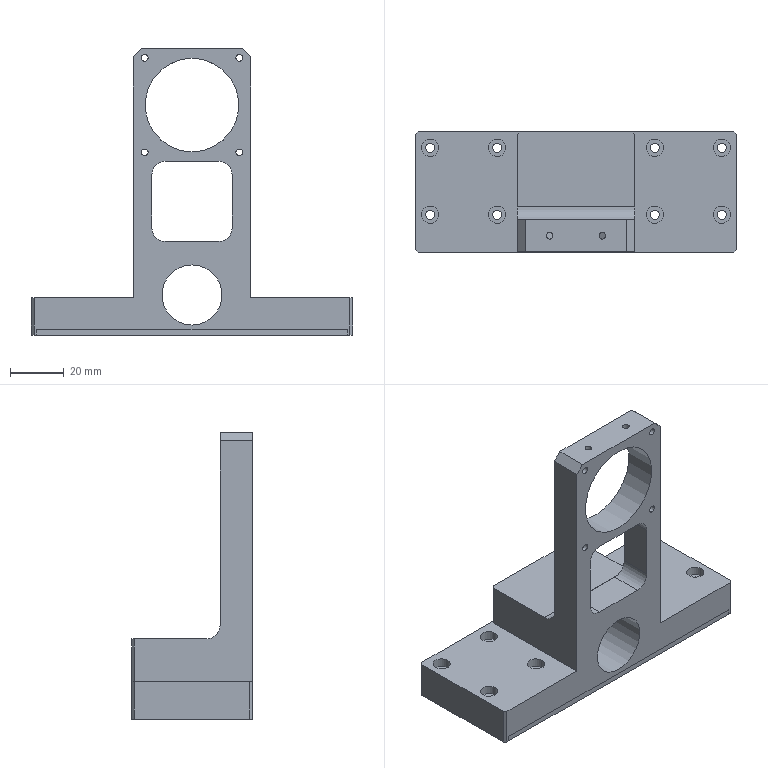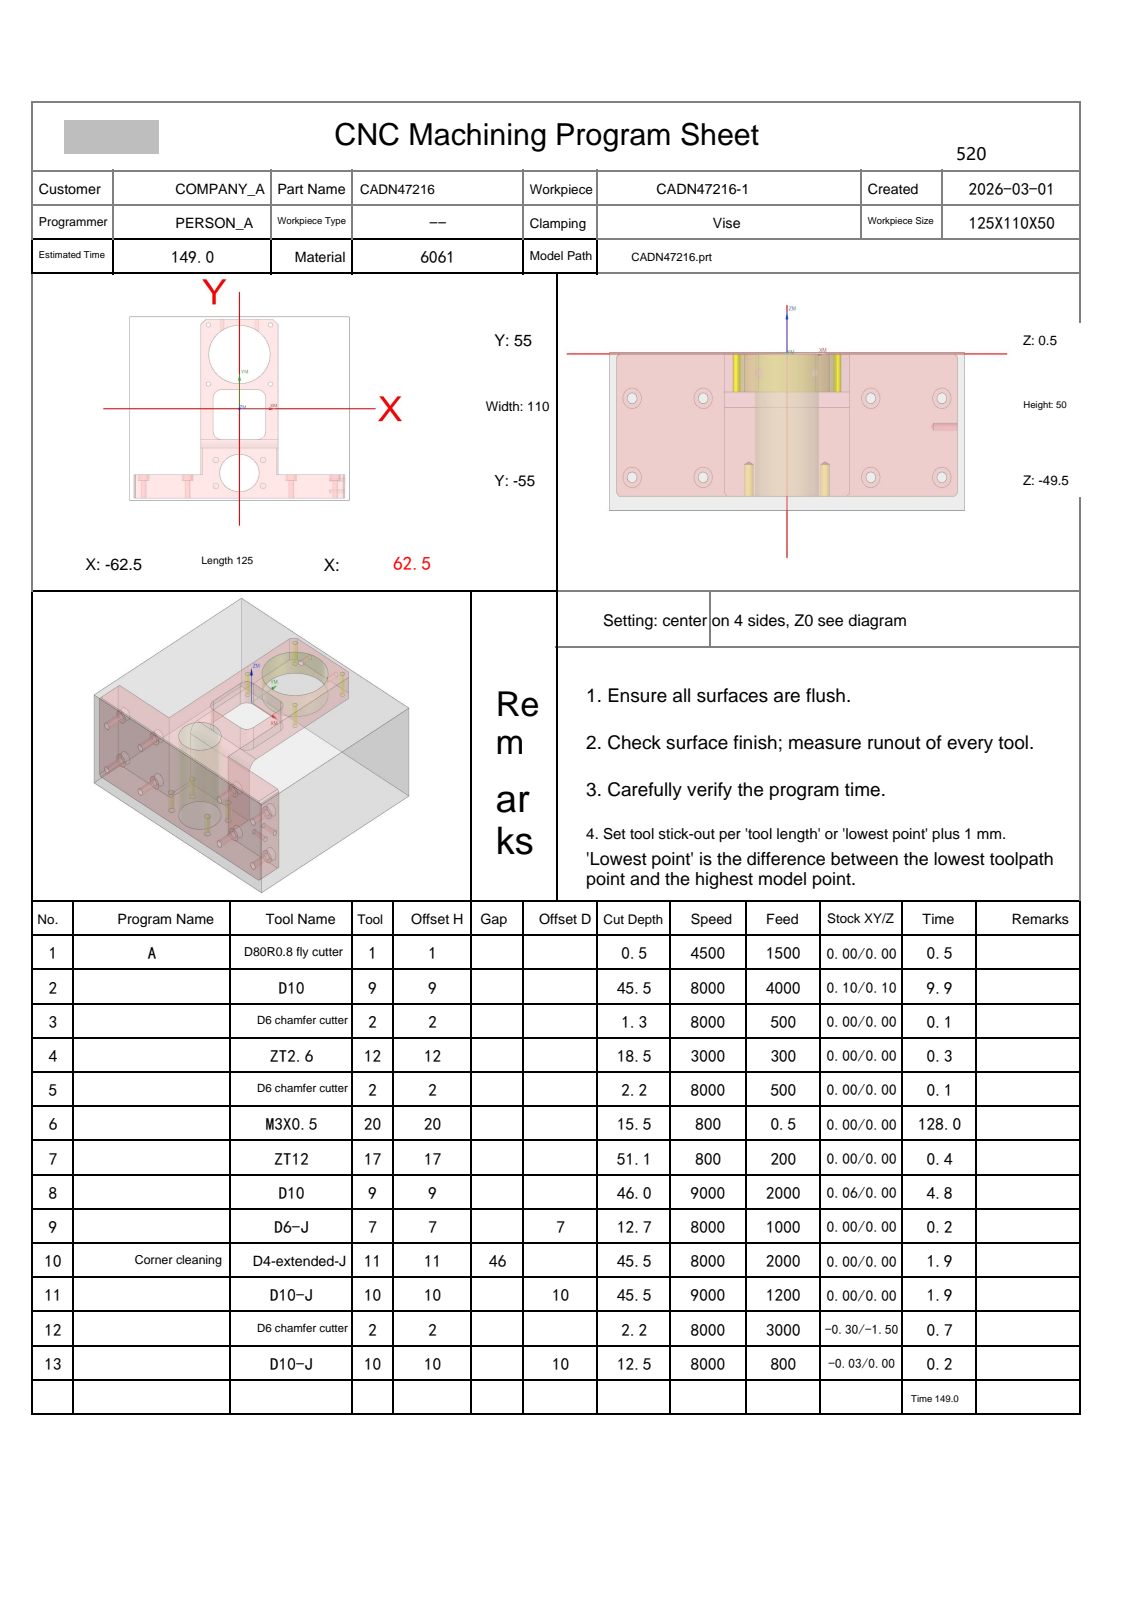NC program | NX | posted by the shop | part box 120 x 45 x 107 mm
Lines 40 to 824 of 16292:
N2 T09 M06
(D10  D=10. R=0. H=09 ce=0.10 di=0.10)
G00 G90 G54 X.938 Y-66.481 M03 S8000
G43 H09 Z50.
M08
Z-13.
G01 X.919 Y-66.382 Z-13.625 F4000.
X.9 Y-66.284 Z-13.872
X.882 Y-66.186 Z-14.054
X.863 Y-66.088 Z-14.2
X.844 Y-65.989 Z-14.323
X.826 Y-65.891 Z-14.428
X.807 Y-65.793 Z-14.52
X.788 Y-65.695 Z-14.6
X.77 Y-65.596 Z-14.67
X.751 Y-65.498 Z-14.732
X.732 Y-65.4 Z-14.786
X.713 Y-65.302 Z-14.833
X.695 Y-65.203 Z-14.874
X.676 Y-65.105 Z-14.908
X.657 Y-65.007 Z-14.936
X.639 Y-64.909 Z-14.96
X.62 Y-64.81 Z-14.977
X.601 Y-64.712 Z-14.99
X.583 Y-64.614 Z-14.997
X.564 Y-64.516 Z-15.
X.162 Y-62.401
G03 X-.097 Y-62.05 I-.505 J-.101
X-3.905 Y-61.412 I-4.018 J-12.303
X-14.072 Y-61.231 I-10.167 J-284.631
X-17.398 Y-61.25 I0.0 J-284.813
G01 X-60.678 Y-61.231
G02 X-67.395 Y-56.529 I.013 J7.167
X-68.578 Y-50.351 I18.107 J6.671
X-68.773 Y-39.514 I302.203 J10.837
X-68.75 Y-35.794 I302.397 J0.0
G01 X-68.728 Y53.226
G02 X-63.998 Y59.919 I7.18 J-.057
X-57.815 Y61.083 I6.651 J-18.335
X-47.788 Y61.267 I10.027 J-273.084
X-44.698 Y61.249 I0.0 J-273.268
G01 X60.642 Y61.232
X60.679
G02 X67.342 Y56.649 I0.0 J-7.136
X68.57 Y50.481 I-17.504 J-6.69
X68.762 Y41.34 I-217.868 J-9.141
X68.749 Y38.964 I-218.06 J0.0
G01 X68.727 Y-53.256
G02 X64.061 Y-59.88 I-7.149 J.08
X58.045 Y-61.066 I-6.6 J17.634
X48.918 Y-61.262 I-9.127 J212.083
X46.528 Y-61.249 I0.0 J212.279
G01 X2.708 Y-61.234
G03 X-4.185 Y-60.645 I-44.506 J-480.047
X-14.751 Y-60.443 I-10.567 J-276.355
X-16.677 Y-60.45 I0.0 J-276.557
G01 X-58.817 Y-60.43
G02 X-65.806 Y-56.095 I.112 J7.983
X-67.58 Y-49.824 I14.829 J7.58
X-67.956 Y-40.805 I107.884 J9.02
X-67.943 Y-39.115 I108.261 J0.0
G01 X-67.927 Y51.377
G02 X-63.534 Y58.349 I7.983 J-.16
X-57.088 Y60.108 I7.633 J-15.278
X-48.536 Y60.448 I8.552 J-107.301
X-47.258 Y60.441 I0.0 J-107.641
G01 X58.897 Y60.426
G02 X65.869 Y55.979 I-.204 J-8.008
X67.586 Y49.773 I-15.088 J-7.514
X67.95 Y41.089 I-103.204 J-8.684
X67.941 Y39.703 I-103.569 J0.0
G01 X67.926 Y-51.397
G02 X63.72 Y-58.236 I-7.953 J.178
X57.616 Y-60.051 I-7.424 J13.793
X48.804 Y-60.452 I-8.811 J96.695
X47.308 Y-60.44 I0.0 J97.096
G01 X4.129 Y-60.424
G02 X-4.091 Y-59.876 I46.615 J762.033
G03 X-16.229 Y-59.643 I-12.138 J-315.046
X-18.439 Y-59.65 I0.0 J-315.28
G01 X-57.058 Y-59.629
G02 X-61.6 Y-58.31 I.078 J8.75
G01 X-62.55 Y-57.917
X-63.606 Y-57.106
G02 X-65.914 Y-52.612 I8.884 J7.4
X-67.005 Y-44.788 I31.157 J8.335
X-67.162 Y-33.373 I415.458 J11.415
X-67.149 Y-30.07 I415.615 J0.0
G01 X-67.126 Y49.59
G02 X-62.035 Y57.472 I8.98 J-.215
X-55.352 Y59.266 I8.136 J-16.972
X-46.19 Y59.648 I9.162 J-109.56
X-44.803 Y59.639 I0.0 J-109.942
G01 X57.097 Y59.626
G02 X64.995 Y54.479 I-.239 J-9.002
X66.78 Y47.704 I-17.291 J-8.176
X67.147 Y38.63 I-111.949 J-9.074
X67.139 Y37.314 I-112.316 J0.0
G01 X67.125 Y-49.626
G02 X64.575 Y-55.668 I-8.841 J.172
G01 X64.417 Y-56.05
X63.606 Y-57.106
X62.55 Y-57.917
G02 X59.208 Y-58.876 I-4.729 J10.179
X49.323 Y-59.623 I-9.884 J64.963
X48.606 Y-59.619 I0.0 J65.711
G01 X6.626 Y-59.644
G02 X-3.614 Y-59.12 I6.006 J217.923
G03 X-18.604 Y-58.832 I-14.991 J-389.723
X-22.439 Y-58.851 I0.0 J-390.011
G01 X-55.378 Y-58.826
G02 X-57.37 Y-58.6 I1.372 J20.951
G01 X-60.002
X-61.32 Y-58.426
X-62.55 Y-57.917
X-63.606 Y-57.106
X-64.417 Y-56.05
X-64.926 Y-54.82
G03 X-65.756 Y-49.323 I-665.252 J-97.63
G02 X-66.324 Y-39.106 I91.575 J10.217
X-66.322 Y-38.384 I92.143 J0.0
G01 X-66.34 Y47.356
G02 X-66.345 Y47.678 I9.923 J.322
X-63.798 Y54.318 I9.929 J0.0
X-57.412 Y57.808 I9.095 J-9.055
X-49.08 Y58.744 I8.629 J-39.28
X-37.639 Y58.852 I11.442 J-603.313
X-35.481 Y58.848 I0.0 J-603.421
G01 X55.379 Y58.823
G02 X64.126 Y53.152 I-.126 J-9.775
X65.968 Y45.982 I-18.796 J-8.65
X66.349 Y36.35 I-121.618 J-9.633
X66.34 Y34.873 I-121.998 J0.0
G01 X66.326 Y-47.827
G02 X65.114 Y-52.678 I-11.697 J.345
G01 Y-52.741
G02 X64.926 Y-54.82 I-11.608 J0.0
G01 X64.559 Y-55.707
X64.926 Y-54.82
G03 X65.118 Y-52.554 I-13.274 J2.266
G01 X65.117 Y-52.404
G03 X65.694 Y-44.314 I-56.506 J8.09
X65.688 Y-43.513 I-57.083 J0.0
G01 X65.693 Y35.681
G03 X65.7 Y36.803 I-96.235 J1.122
X65.253 Y46.067 I-96.241 J0.0
X63.29 Y52.784 I-17.961 J-1.602
X56.295 Y57.642 I-8.568 J-4.871
X49.549 Y58.185 I-6.746 J-41.703
X48.885 Y58.179 I0.0 J-42.245
G01 X20.867 Y58.216
X20.32 Y58.426
X19.002 Y58.6
X-18.998
G02 X-25.006 Y58.226 I-6.008 J48.111
X-25.702 Y58.231 I0.0 J48.485
G01 X-46.041 Y58.164
G03 X-46.411 Y58.165 I-.37 J-59.275
X-55.208 Y57.508 I0.0 J-59.276
X-61.478 Y55.005 I2.062 J-14.27
X-65.17 Y48.656 I6.192 J-7.848
X-65.685 Y41.954 I43.364 J-6.702
X-65.68 Y41.323 I43.879 J0.0
G01 X-65.706 Y-31.857
G03 X-65.722 Y-34.468 I211.033 J-2.611
X-65.419 Y-45.771 I211.049 J0.0
G01 X-65.1 Y-49.022
Y-53.498
X-65.082 Y-39.261
G03 X-64.891 Y-30.437 I-203.923 J8.824
X-64.909 Y-27.741 I-204.113 J0.0
G01 X-64.886 Y40.059
G02 X-64.892 Y40.79 I47.066 J.732
X-64.437 Y47.317 I47.072 J0.0
X-57.999 Y55.432 I10.346 J-1.597
X-50.691 Y57.075 I8.716 J-21.695
X-40.602 Y57.413 I10.089 J-150.449
X-38.778 Y57.402 I0.0 J-150.787
G03 X-34.503 Y57.384 I4.276 J507.053
X-22.81 Y57.519 I0.0 J507.071
G01 X-22.664 Y57.514
G03 X-21.902 Y57.646 I0.0 J2.257
G01 X-21.55 Y57.917
X-20.32 Y58.426
X-20.082 Y58.458
G03 X-22.034 Y57.557 I.936 J-4.594
G02 X-25.711 Y56.931 I-3.835 J11.422
X-35.308 Y56.749 I-9.596 J251.889
X-37.987 Y56.763 I0.0 J252.071
G03 X-39.995 Y56.776 I-2.008 J-149.652
X-50.219 Y56.427 I0.0 J-149.666
X-57.284 Y54.802 I1.358 J-22.08
X-63.375 Y47.391 I4.336 J-9.773
X-64.2 Y39.981 I32.884 J-7.41
G01 Y39.853
G03 X-64.268 Y30.725 I610.552 J-9.128
G01 Y30.414
X-64.29 Y-33.775
G02 X-64.286 Y-34.277 I-34.599 J-.501
X-64.384 Y-36.876 I-34.603 J0.0
G01 X-64.926 Y-38.177
X-65.1 Y-39.493
X-64.926 Y-38.177
G03 X-64.056 Y-36.014 I-17.431 J8.264
X-63.536 Y-30.602 I-27.9 J5.412
G01 X-63.537 Y-30.434
G03 X-63.467 Y-20.91 I-645.856 J9.524
X-63.468 Y-19.342 I-645.927 J0.0
G01 X-63.441 Y36.938
G02 X-63.445 Y37.587 I51.623 J.648
X-62.911 Y44.992 I51.627 J0.0
X-59.625 Y51.611 I11.541 J-1.605
X-53.053 Y54.935 I9.391 J-10.406
X-44.317 Y55.864 I9.056 J-43.619
X-29.665 Y56.012 I16.625 J-921.263
G03 X-29.307 Y56.01 I.357 J34.049
X-23.651 Y56.483 I0.0 J34.051
X-22.605 Y57.107 I-.191 J1.509
G01 X-21.907 Y57.643
G03 X-23.124 Y56.599 I5.322 J-7.436
G02 X-26.2 Y55.709 I-3.698 J7.028
X-33.987 Y55.328 I-7.787 J79.357
X-35.051 Y55.335 I0.0 J79.738
G03 X-36.85 Y55.345 I-1.799 J-176.429
X-47.839 Y55.002 I0.0 J-176.438
X-55.228 Y53.373 I1.312 J-23.522
X-61.749 Y45.734 I4.493 J-10.437
X-62.716 Y38.376 I30.263 J-7.72
X-62.833 Y28.23 I440.37 J-10.146
X-62.828 Y26.217 I440.487 J0.0
G01 X-62.854 Y-27.449
G02 X-62.849 Y-28.175 I-50.354 J-.726
X-63.278 Y-34.736 I-50.359 J0.0
X-63.607 Y-35.893 I-3.31 J.316
G01 X-64.386 Y-36.909
G03 X-63.206 Y-35.305 I-9.361 J8.126
X-62.311 Y-31.179 I-11.97 J4.756
X-62.018 Y-22.096 I-140.689 J9.083
X-62.03 Y-20.218 I-140.982 J0.0
G01 X-62.001 Y33.918
G02 X-62.006 Y34.649 I58.66 J.731
X-61.452 Y42.692 I58.664 J0.0
X-58.71 Y49.173 I13.186 J-1.759
X-52.046 Y53.231 I9.896 J-8.751
X-43.342 Y54.38 I9.291 J-36.821
X-31.156 Y54.609 I22.713 J-885.813
G03 X-25.062 Y55.253 I-.047 J29.593
X-24.119 Y55.593 I-1.278 J5.023
G01 X-23.044 Y56.668
G02 X-24.408 Y55.361 I-11.057 J10.172
X-28.039 Y54.311 I-4.438 J8.545
X-36.558 Y53.879 I-8.52 J83.818
X-37.005 Y53.881 I0.0 J84.25
G03 X-37.589 Y53.882 I-.584 J-96.774
X-47.627 Y53.36 I0.0 J-96.775
X-54.704 Y51.228 I1.865 J-19.001
X-60.224 Y43.912 I6.084 J-10.331
X-61.262 Y36.24 I31.27 J-8.136
X-61.396 Y25.662 I416.43 J-10.578
X-61.388 Y23.041 I416.564 J0.0
G01 X-61.415 Y-24.01
G02 X-61.411 Y-24.739 I-60.766 J-.729
X-61.893 Y-32.38 I-60.77 J0.0
X-62.751 Y-35.211 I-8.826 J1.128
G01 X-63.607 Y-35.893
G03 X-62.331 Y-34.756 I-2.769 J4.392
X-61.13 Y-31.04 I-8.433 J4.776
X-60.615 Y-22.722 I-66.874 J8.319
X-60.619 Y-22.018 I-67.389 J0.0
G01 X-60.588 Y-12.782
X-60.56 Y31.418
G02 X-60.565 Y32.138 I63.191 J.72
X-59.996 Y40.592 I63.195 J0.0
X-57.316 Y47.284 I14.324 J-1.856
X-50.478 Y51.686 I10.276 J-8.451
X-42.346 Y52.891 I9.197 J-34.014
G01 X-31.65 Y53.244
G03 X-25.868 Y54.12 I-.494 J22.785
G01 X-25.372 Y54.341
X-24.127 Y55.585
G02 X-25.651 Y54.107 I-33.884 J33.399
X-29.388 Y52.948 I-4.692 J8.531
X-38.113 Y52.407 I-9.396 J80.902
G03 X-47.511 Y51.626 I.39 J-61.558
X-54.468 Y48.722 I2.449 J-15.658
X-58.862 Y41.643 I8.267 J-10.034
X-59.843 Y33.399 I36.579 J-8.534
X-59.95 Y22.664 I538.974 J-10.735
X-59.948 Y21.08 I539.081 J0.0
G01 X-59.974 Y-21.132
G02 X-59.969 Y-21.92 I-71.71 J-.787
X-60.484 Y-30.494 I-71.714 J0.0
X-61.745 Y-34.504 I-10.691 J1.158
X-62.552 Y-35.084 I-1.081 J.654
G01 X-62.742 Y-35.23
G02 X-61.958 Y-34.832 I1.679 J-2.338
G03 X-60.457 Y-32.518 I-3.047 J3.62
X-59.385 Y-26.183 I-22.771 J7.112
X-59.141 Y-15.865 I-218.36 J10.318
X-59.148 Y-14.061 I-218.604 J0.0
G01 X-59.122 Y28.878
G02 X-59.126 Y29.645 I69.952 J.767
X-58.57 Y38.454 I69.956 J0.0
X-56.033 Y45.291 I15.608 J-1.903
X-49.081 Y50.104 I10.656 J-7.963
X-40.569 Y51.452 I9.672 J-33.525
G03 X-31.276 Y51.979 I-8.574 J233.462
X-26.442 Y53.103 I-1.002 J15.262
X-25.605 Y54.107 I-3.408 J3.692
G01 X-25.379 Y54.334
G03 X-26.384 Y53.103 I12.321 J-11.088
G02 X-29.43 Y51.804 I-4.205 J5.638
X-36.304 Y51.045 I-8.22 J42.929
G03 X-45.295 Y50.25 I2.324 J-77.557
X-52.417 Y47.511 I2.442 J-16.98
X-57.275 Y40.271 I7.828 J-10.502
X-58.359 Y32.364 I33.322 J-8.599
X-58.519 Y21.282 I384.967 J-11.082
X-58.508 Y18.365 I385.127 J0.0
G01 X-58.533 Y-18.734
G02 X-58.529 Y-19.548 I-81.428 J-.814
X-59.062 Y-28.846 I-81.432 J0.0
X-60.44 Y-33.545 I-13.681 J1.461
X-61.261 Y-34.553 I-2.398 J1.115
G01 X-62.082 Y-34.889
G03 X-60.842 Y-34.337 I-1.711 J5.511
X-59.097 Y-31.486 I-4.232 J4.548
X-57.953 Y-24.51 I-26.426 J7.916
X-57.7 Y-13.635 I-233.718 J10.875
X-57.708 Y-11.741 I-233.971 J0.0
G01 X-57.676 Y27.178
G02 X-57.68 Y27.854 I66.822 J.676
X-57.063 Y36.91 I66.826 J0.0
X-54.415 Y43.799 I15.78 J-2.112
X-47.206 Y48.692 I10.931 J-8.349
X-39.173 Y50.022 I9.948 J-35.162
G03 X-31.169 Y50.76 I-5.104 J99.11
X-27.062 Y52.061 I-1.413 J11.592
X-26.682 Y52.41 I-.803 J1.256
G02 X-26.319 Y53.177 I3.349 J-1.114
G03 X-26.75 Y52.265 I4.395 J-2.634
G02 X-29.107 Y50.832 I-3.746 J3.507
X-35.282 Y49.721 I-7.866 J26.016
G03 X-43.668 Y48.79 I6.364 J-95.529
X-50.835 Y45.983 I2.667 J-17.36
X-55.836 Y38.439 I8.119 J-10.812
X-56.935 Y29.969 I36.102 J-8.992
X-57.078 Y18.488 I463.187 J-11.481
X-57.068 Y15.49 I463.329 J0.0
G01 X-57.093 Y-16.656
G02 X-57.09 Y-17.474 I-90.058 J-.818
X-57.641 Y-27.426 I-90.062 J0.0
X-59.238 Y-32.927 I-15.669 J1.567
X-60.62 Y-34.47 I-3.453 J1.7
G01 X-61.313 Y-34.573
G03 X-59.205 Y-33.454 I-.017 J2.576
X-57.287 Y-28.974 I-8.928 J6.473
X-56.382 Y-19.934 I-48.272 J9.401
X-56.268 Y-9.022 I-621.468 J11.921
G01 X-56.239 Y24.798
G02 X-56.242 Y25.483 I75.248 J.685
X-55.676 Y34.695 I75.251 J0.0
X-53.134 Y41.878 I17.133 J-2.023
X-45.832 Y47.142 I11.302 J-7.981
X-38.144 Y48.607 I10.728 J-35.396
G03 X-30.911 Y49.626 I-4.783 J60.098
X-27.274 Y51.184 I-1.792 J9.207
X-26.926 Y51.82 I-.435 J.651
G01 X-26.712 Y52.337
G03 X-26.984 Y51.464 I2.362 J-1.214
G02 X-29.029 Y49.849 I-3.565 J2.413
X-34.852 Y48.4 I-8.023 J19.823
G03 X-42.704 Y47.225 I11.217 J-101.754
X-49.827 Y44.044 I3.132 J-16.584
X-54.399 Y36.651 I9.094 J-10.733
X-55.492 Y28.099 I37.346 J-9.119
X-55.638 Y16.421 I466.496 J-11.678
X-55.628 Y13.301 I466.642 J0.0
G01 X-55.661 Y-15.527
G02 X-55.659 Y-16.188 I-87.093 J-.661
X-56.292 Y-26.668 I-87.096 J0.0
X-58.028 Y-32.447 I-16.801 J1.899
X-59.794 Y-34.373 I-4.213 J2.091
G01 X-60.638 Y-34.484
G03 X-59.385 Y-34.263 I-.096 J4.22
X-57.158 Y-31.748 I-2.808 J4.73
X-55.419 Y-25.268 I-18.222 J8.361
X-54.858 Y-14.553 I-101.954 J10.715
X-54.859 Y-14.022 I-102.515 J0.0
G01 X-54.792 Y23.358
G02 X-54.794 Y23.912 I70.999 J.554
X-54.178 Y33.251 I71.001 J0.0
X-51.469 Y40.541 I17.021 J-2.176
X-44.194 Y45.709 I11.494 J-8.474
X-37.247 Y47.226 I12.036 J-38.469
G03 X-30.503 Y48.598 I-4.766 J40.682
X-27.234 Y50.496 I-1.985 J7.181
G01 X-27.06 Y50.807
X-26.955 Y51.601
G02 X-27.18 Y50.459 I-3.421 J.08
X-29.503 Y48.585 I-4.328 J2.988
X-35.354 Y46.937 I-9.21 J21.495
G03 X-42.772 Y45.38 I9.388 J-63.162
X-50.018 Y40.83 I3.915 J-14.28
X-53.293 Y33.509 I12.835 J-10.136
X-54.114 Y24.197 I53.029 J-9.366
X-54.192 Y13.818 I693.149 J-10.38
X-54.188 Y11.398 I693.227 J0.0
G01 X-54.215 Y-13.215
G02 X-54.212 Y-14.002 I-103.434 J-.787
X-54.812 Y-25.127 I-103.437 J0.0
X-56.6 Y-31.673 I-20.388 J2.05
X-58.925 Y-34.33 I-5.499 J2.467
X-59.56 Y-34.424 I-.635 J2.098
X-59.885 Y-34.4 I0.0 J2.192
G03 X-59.52 Y-34.423 I.365 J2.843
X-57.292 Y-33.36 I0.0 J2.866
X-54.877 Y-28.705 I-8.334 J7.277
X-53.641 Y-20.14 I-38.495 J9.925
X-53.374 Y-7.288 I-308.186 J12.852
X-53.388 Y-4.301 I-308.454 J0.0
G01 X-53.352 Y21.439
G02 X-53.354 Y22.025 I72.507 J.586
X-52.723 Y31.57 I72.509 J0.0
X-49.968 Y39.006 I17.42 J-2.227
X-42.733 Y44.26 I11.858 J-8.72
X-35.317 Y46.114 I16.643 J-50.814
G03 X-29.407 Y47.959 I-3.984 J23.152
X-27.161 Y49.818 I-2.396 J5.182
X-27.068 Y50.74 I-4.935 J.96
G01 X-27.11 Y49.872
G02 X-28.895 Y47.868 I-3.807 J1.595
X-34.09 Y45.831 I-8.812 J14.828
G03 X-41.169 Y44.023 I22.975 J-104.745
X-48.214 Y39.675 I4.436 J-15.068
X-51.792 Y32.094 I12.454 J-10.511
X-52.673 Y22.412 I52.738 J-9.682
G01 Y22.388
G03 X-52.752 Y11.94 I692.468 J-10.448
X-52.748 Y9.589 I692.547 J0.0
G01 X-52.781 Y-12.249
G02 X-52.78 Y-12.848 I-102.91 J-.598
X-53.429 Y-24.391 I-102.912 J0.0
X-55.298 Y-31.219 I-22.09 J2.377
X-57.836 Y-34.233 I-6.469 J2.871
G01 X-58.261 Y-34.4
X-59.061
G03 X-58.663 Y-34.422 I.398 J3.525
X-57.55 Y-34.243 I0.0 J3.547
X-54.967 Y-31.635 I-2.894 J5.448
X-52.86 Y-25.184 I-17.102 J9.156
X-52.018 Y-13.585 I-79.799 J11.622
X-51.944 Y-3.438 I-691.039 J10.148
X-51.948 Y-1.022 I-691.113 J0.0
G01 X-51.913 Y19.498
G02 X-51.915 Y20.11 I75.303 J.611
X-51.28 Y29.87 I75.305 J0.0
X-48.587 Y37.334 I18.063 J-2.299
X-41.568 Y42.75 I12.282 J-8.661
X-34.587 Y44.874 I21.032 J-56.584
G03 X-29.054 Y47.077 I-4.677 J19.796
X-27.133 Y48.984 I-2.775 J4.716
X-27.097 Y49.798 I-9.154 J.814
X-27.1 Y50.011 I-9.19 J0.0
G02 X-27.079 Y49.611 I-3.87 J-.4
X-27.173 Y48.763 I-3.89 J0.0
X-29.363 Y46.461 I-4.777 J2.354
X-34.844 Y44.216 I-11.077 J19.227
G03 X-41.438 Y41.992 I13.56 J-51.074
X-49.968 Y31.993 I5.823 J-13.605
X-51.151 Y23.131 I38.059 J-9.591
X-51.321 Y10.967 I435.224 J-12.164
X-51.308 Y7.612 I435.393 J0.0
G02 X-51.283 Y1.032 I-874.496 J-6.581
X-51.444 Y-15.758 I-874.521 J0.0
X-52.491 Y-26.266 I-61.083 J.776
X-54.881 Y-32.337 I-16.469 J2.979
X-57.194 Y-34.386 I-4.734 J3.014
G01 X-58.16 Y-34.4
G03 X-57.724 Y-34.424 I.436 J3.927
X-56.569 Y-34.252 I0.0 J3.951
X-53.818 Y-31.563 I-2.904 J5.724
X-51.514 Y-24.764 I-17.554 J9.74
X-50.599 Y-13.204 I-77.325 J11.935
X-50.486 Y1.037 I-897.128 J14.241
X-50.508 Y7.359 I-897.241 J0.0
G02 X-50.529 Y11.088 I336.414 J3.729
X-50.294 Y23.655 I336.435 J0.0
X-48.9 Y32.156 I32.597 J-.98
X-40.958 Y41.024 I14.109 J-4.645
X-34.369 Y43.508 I22.493 J-49.695
G03 X-29.054 Y45.951 I-6.127 J20.329
X-27.113 Y48.056 I-2.799 J4.529
G01 X-27.1 Y49.1
G02 X-27.081 Y48.669 I-4.928 J-.431
X-27.163 Y47.771 I-4.947 J0.0
X-29.275 Y45.356 I-5.022 J2.26
X-34.503 Y42.861 I-12.368 J19.195
G03 X-40.96 Y40.169 I14.324 J-43.453
X-48.527 Y30.396 I7.3 J-13.468
X-49.701 Y21.611 I38.692 J-9.641
X-49.882 Y9.244 I423.184 J-12.367
X-49.868 Y5.773 I423.364 J0.0
G02 X-49.844 Y.265 I-631.411 J-5.508
X-50.04 Y-15.494 I-631.435 J0.0
X-51.197 Y-26.06 I-58.924 J1.105
X-53.738 Y-32.271 I-16.959 J3.312
X-56.179 Y-34.389 I-4.91 J3.193
G01 X-57.121 Y-34.4
G03 X-56.686 Y-34.423 I.434 J4.036
X-55.527 Y-34.254 I0.0 J4.06
X-52.684 Y-31.557 I-2.93 J5.935
X-50.19 Y-24.516 I-17.716 J10.238
X-49.175 Y-12.598 I-75.71 J12.449
X-49.043 Y2.995 I-923.31 J15.593
X-49.065 Y9.338 I-923.441 J0.0
G02 X-49.081 Y11.908 I204.317 J2.57
X-48.762 Y23.332 I204.333 J0.0
X-47.112 Y31.538 I28.229 J-1.406
X-39.684 Y39.644 I14.426 J-5.762
X-33.229 Y42.494 I33.044 J-66.115
G03 X-28.362 Y45.34 I-6.195 J16.178
X-27.108 Y46.995 I-2.84 J3.456
G01 X-27.1 Y48.079
G02 X-27.082 Y47.626 I-5.912 J-.453
X-27.158 Y46.684 I-5.93 J0.0
X-29.376 Y44.058 I-5.472 J2.371
X-34.587 Y41.295 I-15.369 J22.691
G03 X-40.769 Y38.083 I13.032 J-32.636
X-47.08 Y28.865 I9.184 J-13.058
X-48.265 Y19.842 I39.98 J-9.84
X-48.442 Y7.168 I454.866 J-12.674
X-48.428 Y3.604 I455.042 J0.0
G02 X-48.406 Y-.748 I-435.726 J-4.351
X-48.668 Y-15.85 I-435.748 J0.0
X-50.057 Y-26.502 I-52.993 J1.497
X-52.842 Y-32.565 I-15.978 J3.667
X-55.093 Y-34.385 I-4.692 J3.501
G01 X-56.143 Y-34.4
G03 X-55.679 Y-34.423 I.464 J4.766
X-54.493 Y-34.273 I0.0 J4.788
X-51.677 Y-31.773 I-2.711 J5.889
X-49. Y-24.947 I-16.581 J10.44
X-47.8 Y-13.51 I-65.153 J12.619
X-47.604 Y3.558 I-741.925 J17.069
X-47.623 Y8.879 I-742.122 J0.0
G02 X-47.637 Y11.11 I170.312 J2.231
X-47.263 Y22.39 I170.326 J0.0
X-45.424 Y30.631 I26.673 J-1.627
X-38.412 Y38.331 I15.057 J-6.67
X-32.379 Y41.438 I51.679 J-92.939
G03 X-27.951 Y44.554 I-6.568 J14.039
X-27.1 Y45.877 I-2.421 J2.492
G01 Y46.997
G02 X-27.079 Y46.499 I-6.04 J-.498
X-27.162 Y45.504 I-6.06 J0.0
X-29.282 Y42.845 I-5.773 J2.429
X-33.928 Y40.013 I-17.118 J22.855
G03 X-40.042 Y36.27 I14.759 J-30.977
X-45.793 Y26.761 I10.905 J-13.088
X-46.851 Y17.557 I45.715 J-9.915
X-47.012 Y1.603 I790.769 J-15.953
X-46.996 Y-3.318 I790.929 J0.0
G02 X-46.989 Y-4.982 I-184.322 J-1.664
X-47.531 Y-19.103 I-184.33 J0.0
X-49.427 Y-28.412 I-37.171 J2.724
X-52.558 Y-33.462 I-12.062 J3.983
X-54.074 Y-34.4 I-2.828 J2.878
G01 X-55.034
G03 X-54.563 Y-34.424 I.471 J4.681
X-53.371 Y-34.27 I0.0 J4.705
X-50.412 Y-31.63 I-2.84 J6.16
X-47.647 Y-24.611 I-17.367 J10.897
X-46.376 Y-12.862 I-66.259 J13.106
X-46.162 Y4.415 I-695.105 J17.278
X-46.177 Y9.041 I-695.319 J0.0
G02 X-46.187 Y10.666 I136.056 J1.625
X-45.748 Y21.589 I136.066 J0.0
X-43.647 Y29.929 I25.078 J-1.882
X-37.153 Y37.081 I15.872 J-7.888
X-31.213 Y40.636 I153.319 J-249.405
G03 X-27.535 Y43.827 I-6.52 J11.231
X-27.1 Y44.658 I-2.28 J1.724
G01 Y45.858
G02 X-27.082 Y45.338 I-7.625 J-.519
X-27.154 Y44.294 I-7.643 J0.0
X-29.157 Y41.599 I-6.025 J2.387
X-34.226 Y38.151 I-23.172 J28.61
G03 X-40.266 Y33.429 I12.811 J-22.613
X-44.531 Y24.492 I14.226 J-12.275
X-45.452 Y14.627 I55.834 J-10.19
X-45.574 Y-.659 I960.073 J-15.286
X-45.568 Y-4.105 I960.194 J0.0
G02 X-45.565 Y-5.111 I-158.024 J-1.006
X-46.202 Y-19.291 I-158.027 J0.0
X-48.32 Y-28.719 I-35.623 J3.052
X-51.545 Y-33.574 I-11.646 J4.235
X-52.946 Y-34.4 I-2.783 J3.121
G01 X-53.986
G03 X-53.487 Y-34.423 I.499 J5.355
X-52.275 Y-34.285 I0.0 J5.378
X-49.39 Y-31.856 I-2.648 J6.072
X-46.452 Y-24.98 I-16.346 J11.051
X-45.011 Y-13.535 I-59.848 J13.346
X-44.729 Y1.949 I-424.069 J15.484
X-44.743 Y5.444 I-424.351 J0.0
G02 X-44.757 Y7.655 I180.937 J2.211
X-44.388 Y19.196 I180.951 J0.0
X-42.551 Y27.767 I28.904 J-1.712
X-36.143 Y35.718 I17.215 J-7.316
X-30.625 Y39.535 I353.377 J-505.019
G03 X-27.316 Y42.862 I-6.797 J10.071
X-27.1 Y43.36 I-3.809 J1.946
G01 Y44.64
G02 X-27.081 Y44.084 I-8.297 J-.556
X-27.154 Y42.988 I-8.315 J0.0
X-29.207 Y40.122 I-6.565 J2.536
X-34.151 Y36.359 I-33.204 J38.497
G03 X-39.968 Y30.736 I13.108 J-19.381
X-43.322 Y21.796 I18.053 J-11.872
X-44.052 Y11.354 I74.32 J-10.442
G01 Y11.19
X-44.187 Y-7.574
G02 X-45.118 Y-21.204 I-105.9 J.389
X-47.591 Y-29.819 I-29.474 J3.8
X-50.795 Y-33.889 I-9.827 J4.44
X-51.793 Y-34.4 I-2.054 J2.78
G01 X-52.833
G03 X-52.345 Y-34.419 I.489 J6.418
X-51.243 Y-34.324 I0.0 J6.436
X-48.369 Y-32.085 I-2.253 J5.856
X-45.286 Y-25.421 I-15.35 J11.146
X-43.638 Y-13.817 I-55.606 J13.819
X-43.291 Y1.748 I-349.007 J15.566
X-43.302 Y4.569 I-349.354 J0.0
G02 X-43.314 Y6.57 I164.856 J2.001
X-42.906 Y18.159 I164.868 J0.0
X-40.833 Y27.08 I28.177 J-1.848
X-34.788 Y34.677 I18.699 J-8.676
G03 X-29.72 Y38.713 I-137.002 J177.224
X-27.121 Y41.875 I-6.339 J7.859
G01 X-27.1 Y43.342
G02 X-27.077 Y42.716 I-8.453 J-.627
X-27.148 Y41.62 I-8.476 J0.0
X-29.097 Y38.702 I-6.96 J2.541
X-33.843 Y34.609 I-49.035 J52.059
G03 X-39.825 Y27.264 I13.831 J-17.374
X-42.177 Y18.171 I25.079 J-11.337
X-42.662 Y6.854 I131.944 J-11.317
X-42.654 Y5.465 I132.428 J0.0
G02 X-42.645 Y2.759 I-374.439 J-2.706
X-43.001 Y-13.571 I-374.449 J0.0
X-44.645 Y-25.215 I-58.587 J2.336
X-47.75 Y-32.048 I-19.304 J4.648
X-50.514 Y-34.379 I-5.844 J4.127
G01 X-51.66 Y-34.4
G03 X-51.161 Y-34.423 I.499 J5.441
X-49.934 Y-34.283 I0.0 J5.464
X-46.947 Y-31.804 I-2.752 J6.355
X-43.859 Y-24.894 I-16.699 J11.607
X-42.217 Y-13.252 I-58.081 J14.129
X-41.844 Y3.255 I-364.992 J16.507
X-41.851 Y5.615 I-365.365 J0.0
G02 X-41.858 Y6.865 I117.134 J1.25
X-41.312 Y18.157 I117.141 J0.0
X-38.697 Y27.259 I25.461 J-2.388
X-33.053 Y34.075 I21.614 J-12.152
G03 X-28.565 Y38.275 I-35.43 J42.362
X-27.113 Y40.447 I-6.043 J5.613
G01 X-27.1 Y41.97
G02 X-27.077 Y41.304 I-9.644 J-.666
X-27.146 Y40.152 I-9.667 J0.0
X-29.048 Y37.116 I-7.527 J2.602
X-33.642 Y32.62 I-104.165 J101.841
G03 X-40.35 Y19.57 I15.862 J-16.401
X-41.161 Y8.73 I72.142 J-10.853
G01 X-41.322 Y-6.285
G02 X-42.349 Y-20.491 I-107.744 J.649
X-44.983 Y-29.536 I-31.357 J4.227
X-48.389 Y-33.863 I-10.498 J4.759
X-49.434 Y-34.4 I-2.348 J3.28
G01 X-50.474
G03 X-49.975 Y-34.423 I.499 J5.472
X-48.737 Y-34.281 I0.0 J5.495
X-45.709 Y-31.781 I-2.8 J6.475
X-42.5 Y-24.647 I-17.05 J11.957
X-40.789 Y-12.609 I-59.703 J14.625
X-40.402 Y3.998 I-355.416 J16.608
X-40.404 Y5.325 I-355.804 J0.0
G02 X-40.407 Y6.164 I102.958 J.838
X-39.786 Y17.462 I102.962 J0.0
X-36.554 Y27.361 I25.023 J-2.691
X-31.379 Y33.599 I27.871 J-17.86
G03 X-27.694 Y37.779 I-19.156 J20.604
X-27.1 Y38.947 I-4.017 J2.776
G01 Y40.467
G02 X-27.084 Y39.821 I-13.571 J-.647
X-27.141 Y38.579 I-13.586 J0.0
X-29.014 Y35.381 I-8.311 J2.72
G01 X-33.371 Y30.501
G03 X-38.959 Y17.967 I18.834 J-15.91
X-39.739 Y6.648 I81.766 J-11.319
G01 Y6.403
G02 X-40.099 Y-11.433 I-472.239 J.614
X-41.773 Y-24.124 I-66.657 J2.336
X-44.997 Y-31.625 I-21.824 J4.938
X-48.102 Y-34.371 I-6.598 J4.332
G01 X-49.274 Y-34.4
G03 X-48.775 Y-34.423 I.499 J5.488
X-47.529 Y-34.28 I0.0 J5.511
X-44.503 Y-31.815 I-2.79 J6.515
X-41.286 Y-24.943 I-16.739 J12.025
X-39.405 Y-12.663 I-57.48 J15.089
X-38.952 Y4.924 I-341.824 J17.588
G01 X-38.953 Y5.177
Y5.575
G02 X-38.225 Y16.987 I89.779 J0.0
X-32.002 Y30.682 I25.538 J-3.343
G03 X-28.057 Y35.473 I-53.812 J48.327
X-27.1 Y37.244 I-5.828 J4.296
G01 Y38.924
G02 X-27.092 Y38.311 I-23.114 J-.613
X-27.136 Y36.882 I-23.122 J0.0
X-28.916 Y33.569 I-9.152 J2.783
G03 X-33.095 Y28.137 I128.391 J-103.096
X-37.587 Y16.27 I22.376 J-15.252
X-38.303 Y5.021 I88.891 J-11.309
G02 X-38.767 Y-12.432 I-351.345 J.609
X-40.672 Y-24.86 I-60.283 J2.877
X-44.008 Y-31.955 I-20.377 J5.25
X-46.972 Y-34.392 I-5.87 J4.12
G01 X-48.137 Y-34.4
G03 X-47.616 Y-34.419 I.522 J7.162
X-46.462 Y-34.326 I0.0 J7.181
X-43.542 Y-32.161 I-2.244 J6.08
X-40.196 Y-25.623 I-15.212 J11.909
X-38.131 Y-14.1 I-51.193 J15.123
X-37.54 Y2.473 I-233.443 J16.623
G01 X-37.541 Y2.861
G02 X-36.928 Y14.691 I114.584 J0.0
X-33. Y26.529 I28.465 J-2.876
X-28.842 Y32.368 I74.885 J-48.92
G03 X-27.118 Y35.29 I-12.287 J9.221
G01 X-27.1 Y37.227
G02 X-27.096 Y36.685 I-37.827 J-.542
X-27.133 Y35.012 I-37.831 J0.0
X-28.676 Y31.786 I-9.847 J2.729
G03 X-32.449 Y26.068 I103.565 J-72.447
X-36.274 Y14.107 I26.502 J-15.068
X-36.901 Y2.063 I115.514 J-12.044
G01 Y2.049
G02 X-37.571 Y-14.728 I-216.087 J.229
X-39.838 Y-26.315 I-49.945 J3.759
X-43.428 Y-32.726 I-17.131 J5.381
X-45.794 Y-34.4 I-4.436 J3.76
G01 X-46.914
G03 X-46.355 Y-34.423 I.559 J6.681
X-45.259 Y-34.333 I0.0 J6.704
X-42.24 Y-32.096 I-2.257 J6.203
X-38.801 Y-25.319 I-15.711 J12.232
X-36.663 Y-13.046 I-54.15 J15.757
X-36.077 Y3.209 I-265.045 J17.691
G02 X-35.259 Y15.092 I88.585 J-.129
X-30.234 Y27.914 I30.983 J-4.746
G03 X-27.3 Y32.797 I-35.433 J24.616
G01 X-27.1 Y33.332
Y35.332
G02 X-27.075 Y34.437 I-16.071 J-.894
X-27.162 Y32.768 I-16.095 J0.0
X-28.835 Y29.111 I-13.797 J4.103
G03 X-32.494 Y22.237 I47.4 J-29.637
X-35.034 Y11.042 I34.64 J-13.747
X-35.526 Y-1.566 I190.821 J-13.757
G02 X-36.525 Y-17.5 I-142.243 J.923
X-39.239 Y-28.074 I-40.249 J4.692
X-42.853 Y-33.368 I-13.756 J5.512
X-44.559 Y-34.4 I-3.407 J3.703
G01 X-45.679
G03 X-45.143 Y-34.423 I.536 J6.205
X-43.88 Y-34.294 I0.0 J6.228
X-40.8 Y-31.876 I-2.728 J6.646
X-37.379 Y-24.946 I-16.81 J12.607
X-35.22 Y-12.318 I-56.716 J16.196
X-34.601 Y3.869 I-313.76 J20.099
G02 X-33.55 Y15.489 I72.7 J-.717